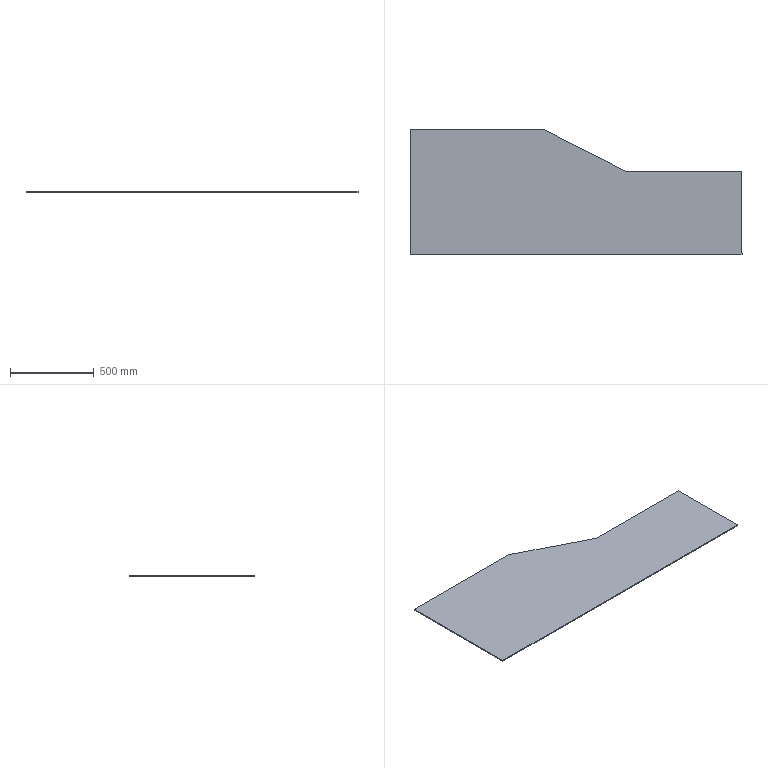Part | SolidWorks | features FlatPattern 1, ICE 1, SMBaseFlange 1, SheetMetal 1 | 1 solid | 8 faces | box 1988 x 750 x 6 mm | volume 7533000 mm3 | plane 8
STEP:
#1=CARTESIAN_POINT('',(-194.,375.,0.));
#2=VERTEX_POINT('',#1);
#3=CARTESIAN_POINT('',(-994.,375.,0.));
#4=VERTEX_POINT('',#3);
#5=CARTESIAN_POINT('',(994.,375.,0.));
#6=DIRECTION('',(-1.,0.,0.));
#7=VECTOR('',#6,1000.);
#8=LINE('',#5,#7);
#9=EDGE_CURVE('',#2,#4,#8,.T.);
#10=ORIENTED_EDGE('',*,*,#9,.F.);
#11=CARTESIAN_POINT('',(-194.,375.,-6.));
#12=VERTEX_POINT('',#11);
#13=CARTESIAN_POINT('',(-194.,375.,0.));
#14=DIRECTION('',(0.,0.,-1.));
#15=VECTOR('',#14,1000.);
#16=LINE('',#13,#15);
#17=EDGE_CURVE('',#2,#12,#16,.T.);
#18=ORIENTED_EDGE('',*,*,#17,.T.);
#19=CARTESIAN_POINT('',(-994.,375.,-6.));
#20=VERTEX_POINT('',#19);
#21=CARTESIAN_POINT('',(994.,375.,-6.));
#22=DIRECTION('',(-1.,0.,0.));
#23=VECTOR('',#22,1000.);
#24=LINE('',#21,#23);
#25=EDGE_CURVE('',#12,#20,#24,.T.);
#26=ORIENTED_EDGE('',*,*,#25,.T.);
#27=CARTESIAN_POINT('',(-994.,375.,-6.));
#28=DIRECTION('',(0.,0.,1.));
#29=VECTOR('',#28,1000.);
#30=LINE('',#27,#29);
#31=EDGE_CURVE('',#20,#4,#30,.T.);
#32=ORIENTED_EDGE('',*,*,#31,.T.);
#33=EDGE_LOOP('',(#10,#18,#26,#32));
#34=FACE_OUTER_BOUND('',#33,.T.);
#35=CARTESIAN_POINT('',(994.,375.,-6.));
#36=DIRECTION('',(0.,1.,0.));
#37=DIRECTION('',(-1.,0.,0.));
#38=AXIS2_PLACEMENT_3D('',#35,#36,#37);
#39=PLANE('',#38);
#40=ADVANCED_FACE('',(#34),#39,.T.);
#41=CARTESIAN_POINT('',(994.,-375.,-6.));
#42=VERTEX_POINT('',#41);
#43=CARTESIAN_POINT('',(994.,125.,-6.));
#44=VERTEX_POINT('',#43);
#45=CARTESIAN_POINT('',(994.,-375.,-6.));
#46=DIRECTION('',(0.,1.,0.));
#47=VECTOR('',#46,1000.);
#48=LINE('',#45,#47);
#49=EDGE_CURVE('',#42,#44,#48,.T.);
#50=ORIENTED_EDGE('',*,*,#49,.T.);
#51=CARTESIAN_POINT('',(994.,125.,0.));
#52=VERTEX_POINT('',#51);
#53=CARTESIAN_POINT('',(994.,125.,0.));
#54=DIRECTION('',(0.,0.,-1.));
#55=VECTOR('',#54,1000.);
#56=LINE('',#53,#55);
#57=EDGE_CURVE('',#52,#44,#56,.T.);
#58=ORIENTED_EDGE('',*,*,#57,.F.);
#59=CARTESIAN_POINT('',(994.,-375.,0.));
#60=VERTEX_POINT('',#59);
#61=CARTESIAN_POINT('',(994.,-375.,0.));
#62=DIRECTION('',(0.,1.,0.));
#63=VECTOR('',#62,1000.);
#64=LINE('',#61,#63);
#65=EDGE_CURVE('',#60,#52,#64,.T.);
#66=ORIENTED_EDGE('',*,*,#65,.F.);
#67=CARTESIAN_POINT('',(994.,-375.,-6.));
#68=DIRECTION('',(0.,0.,1.));
#69=VECTOR('',#68,1000.);
#70=LINE('',#67,#69);
#71=EDGE_CURVE('',#42,#60,#70,.T.);
#72=ORIENTED_EDGE('',*,*,#71,.F.);
#73=EDGE_LOOP('',(#50,#58,#66,#72));
#74=FACE_OUTER_BOUND('',#73,.T.);
#75=CARTESIAN_POINT('',(994.,-375.,-6.));
#76=DIRECTION('',(1.,0.,0.));
#77=DIRECTION('',(0.,0.,-1.));
#78=AXIS2_PLACEMENT_3D('',#75,#76,#77);
#79=PLANE('',#78);
#80=ADVANCED_FACE('',(#74),#79,.T.);
#81=CARTESIAN_POINT('',(298.,125.,-6.));
#82=VERTEX_POINT('',#81);
#83=CARTESIAN_POINT('',(111.635,219.698,-6.));
#84=DIRECTION('',(-0.8915,0.453,0.));
#85=VECTOR('',#84,1000.);
#86=LINE('',#83,#85);
#87=EDGE_CURVE('',#82,#12,#86,.T.);
#88=ORIENTED_EDGE('',*,*,#87,.F.);
#89=CARTESIAN_POINT('',(0.,125.,-6.));
#90=DIRECTION('',(-1.,0.,0.));
#91=VECTOR('',#90,1000.);
#92=LINE('',#89,#91);
#93=EDGE_CURVE('',#44,#82,#92,.T.);
#94=ORIENTED_EDGE('',*,*,#93,.F.);
#95=ORIENTED_EDGE('',*,*,#49,.F.);
#96=CARTESIAN_POINT('',(-994.,-375.,-6.));
#97=VERTEX_POINT('',#96);
#98=CARTESIAN_POINT('',(994.,-375.,-6.));
#99=DIRECTION('',(1.,0.,0.));
#100=VECTOR('',#99,1000.);
#101=LINE('',#98,#100);
#102=EDGE_CURVE('',#97,#42,#101,.T.);
#103=ORIENTED_EDGE('',*,*,#102,.F.);
#104=CARTESIAN_POINT('',(-994.,-375.,-6.));
#105=DIRECTION('',(0.,-1.,0.));
#106=VECTOR('',#105,1000.);
#107=LINE('',#104,#106);
#108=EDGE_CURVE('',#20,#97,#107,.T.);
#109=ORIENTED_EDGE('',*,*,#108,.F.);
#110=ORIENTED_EDGE('',*,*,#25,.F.);
#111=EDGE_LOOP('',(#88,#94,#95,#103,#109,#110));
#112=FACE_OUTER_BOUND('',#111,.T.);
#113=CARTESIAN_POINT('',(0.,0.,-6.));
#114=DIRECTION('',(0.,0.,1.));
#115=DIRECTION('',(1.,0.,0.));
#116=AXIS2_PLACEMENT_3D('',#113,#114,#115);
#117=PLANE('',#116);
#118=ADVANCED_FACE('',(#112),#117,.F.);
#119=CARTESIAN_POINT('',(298.,125.,0.));
#120=VERTEX_POINT('',#119);
#121=CARTESIAN_POINT('',(0.,125.,0.));
#122=DIRECTION('',(-1.,0.,0.));
#123=VECTOR('',#122,1000.);
#124=LINE('',#121,#123);
#125=EDGE_CURVE('',#52,#120,#124,.T.);
#126=ORIENTED_EDGE('',*,*,#125,.T.);
#127=CARTESIAN_POINT('',(111.635,219.698,0.));
#128=DIRECTION('',(-0.8915,0.453,0.));
#129=VECTOR('',#128,1000.);
#130=LINE('',#127,#129);
#131=EDGE_CURVE('',#120,#2,#130,.T.);
#132=ORIENTED_EDGE('',*,*,#131,.T.);
#133=ORIENTED_EDGE('',*,*,#9,.T.);
#134=CARTESIAN_POINT('',(-994.,-375.,0.));
#135=VERTEX_POINT('',#134);
#136=CARTESIAN_POINT('',(-994.,-375.,0.));
#137=DIRECTION('',(0.,-1.,0.));
#138=VECTOR('',#137,1000.);
#139=LINE('',#136,#138);
#140=EDGE_CURVE('',#4,#135,#139,.T.);
#141=ORIENTED_EDGE('',*,*,#140,.T.);
#142=CARTESIAN_POINT('',(994.,-375.,0.));
#143=DIRECTION('',(1.,0.,0.));
#144=VECTOR('',#143,1000.);
#145=LINE('',#142,#144);
#146=EDGE_CURVE('',#135,#60,#145,.T.);
#147=ORIENTED_EDGE('',*,*,#146,.T.);
#148=ORIENTED_EDGE('',*,*,#65,.T.);
#149=EDGE_LOOP('',(#126,#132,#133,#141,#147,#148));
#150=FACE_OUTER_BOUND('',#149,.T.);
#151=CARTESIAN_POINT('',(0.,0.,0.));
#152=DIRECTION('',(0.,0.,1.));
#153=DIRECTION('',(1.,0.,0.));
#154=AXIS2_PLACEMENT_3D('',#151,#152,#153);
#155=PLANE('',#154);
#156=ADVANCED_FACE('',(#150),#155,.T.);
#157=ORIENTED_EDGE('',*,*,#140,.F.);
#158=ORIENTED_EDGE('',*,*,#31,.F.);
#159=ORIENTED_EDGE('',*,*,#108,.T.);
#160=CARTESIAN_POINT('',(-994.,-375.,-6.));
#161=DIRECTION('',(0.,0.,1.));
#162=VECTOR('',#161,1000.);
#163=LINE('',#160,#162);
#164=EDGE_CURVE('',#97,#135,#163,.T.);
#165=ORIENTED_EDGE('',*,*,#164,.T.);
#166=EDGE_LOOP('',(#157,#158,#159,#165));
#167=FACE_OUTER_BOUND('',#166,.T.);
#168=CARTESIAN_POINT('',(-994.,-375.,-6.));
#169=DIRECTION('',(-1.,0.,0.));
#170=DIRECTION('',(0.,0.,1.));
#171=AXIS2_PLACEMENT_3D('',#168,#169,#170);
#172=PLANE('',#171);
#173=ADVANCED_FACE('',(#167),#172,.T.);
#174=ORIENTED_EDGE('',*,*,#146,.F.);
#175=ORIENTED_EDGE('',*,*,#164,.F.);
#176=ORIENTED_EDGE('',*,*,#102,.T.);
#177=ORIENTED_EDGE('',*,*,#71,.T.);
#178=EDGE_LOOP('',(#174,#175,#176,#177));
#179=FACE_OUTER_BOUND('',#178,.T.);
#180=CARTESIAN_POINT('',(994.,-375.,-6.));
#181=DIRECTION('',(0.,-1.,0.));
#182=DIRECTION('',(1.,0.,0.));
#183=AXIS2_PLACEMENT_3D('',#180,#181,#182);
#184=PLANE('',#183);
#185=ADVANCED_FACE('',(#179),#184,.T.);
#186=ORIENTED_EDGE('',*,*,#17,.F.);
#187=ORIENTED_EDGE('',*,*,#131,.F.);
#188=CARTESIAN_POINT('',(298.,125.,0.));
#189=DIRECTION('',(0.,0.,-1.));
#190=VECTOR('',#189,1000.);
#191=LINE('',#188,#190);
#192=EDGE_CURVE('',#120,#82,#191,.T.);
#193=ORIENTED_EDGE('',*,*,#192,.T.);
#194=ORIENTED_EDGE('',*,*,#87,.T.);
#195=EDGE_LOOP('',(#186,#187,#193,#194));
#196=FACE_OUTER_BOUND('',#195,.T.);
#197=CARTESIAN_POINT('',(111.635,219.698,0.));
#198=DIRECTION('',(0.453,0.8915,0.));
#199=DIRECTION('',(-0.8915,0.453,0.));
#200=AXIS2_PLACEMENT_3D('',#197,#198,#199);
#201=PLANE('',#200);
#202=ADVANCED_FACE('',(#196),#201,.T.);
#203=ORIENTED_EDGE('',*,*,#125,.F.);
#204=ORIENTED_EDGE('',*,*,#57,.T.);
#205=ORIENTED_EDGE('',*,*,#93,.T.);
#206=ORIENTED_EDGE('',*,*,#192,.F.);
#207=EDGE_LOOP('',(#203,#204,#205,#206));
#208=FACE_OUTER_BOUND('',#207,.T.);
#209=CARTESIAN_POINT('',(0.,125.,0.));
#210=DIRECTION('',(0.,1.,0.));
#211=DIRECTION('',(-1.,0.,0.));
#212=AXIS2_PLACEMENT_3D('',#209,#210,#211);
#213=PLANE('',#212);
#214=ADVANCED_FACE('',(#208),#213,.T.);
#215=CLOSED_SHELL('',(#40,#80,#118,#156,#173,#185,#202,#214));
#216=MANIFOLD_SOLID_BREP('',#215);
#217=CARTESIAN_POINT('',(0.,0.,0.));
#218=DIRECTION('',(0.,0.,1.));
#219=DIRECTION('',(1.,0.,0.));
#220=AXIS2_PLACEMENT_3D('',#217,#218,#219);
#221=(LENGTH_UNIT()NAMED_UNIT(*)SI_UNIT(.MILLI.,.METRE.));
#222=UNCERTAINTY_MEASURE_WITH_UNIT(LENGTH_MEASURE(0.00001),#221,'','');
#223=(NAMED_UNIT(*)PLANE_ANGLE_UNIT()SI_UNIT($,.RADIAN.));
#224=(NAMED_UNIT(*)SI_UNIT($,.STERADIAN.)SOLID_ANGLE_UNIT());
#225=(GEOMETRIC_REPRESENTATION_CONTEXT(3)GLOBAL_UNCERTAINTY_ASSIGNED_CONTEXT((#222))GLOBAL_UNIT_ASSIGNED_CONTEXT((#221,#223,#224))REPRESENTATION_CONTEXT('',''));
#226=ADVANCED_BREP_SHAPE_REPRESENTATION('',(#216,#220),#225);